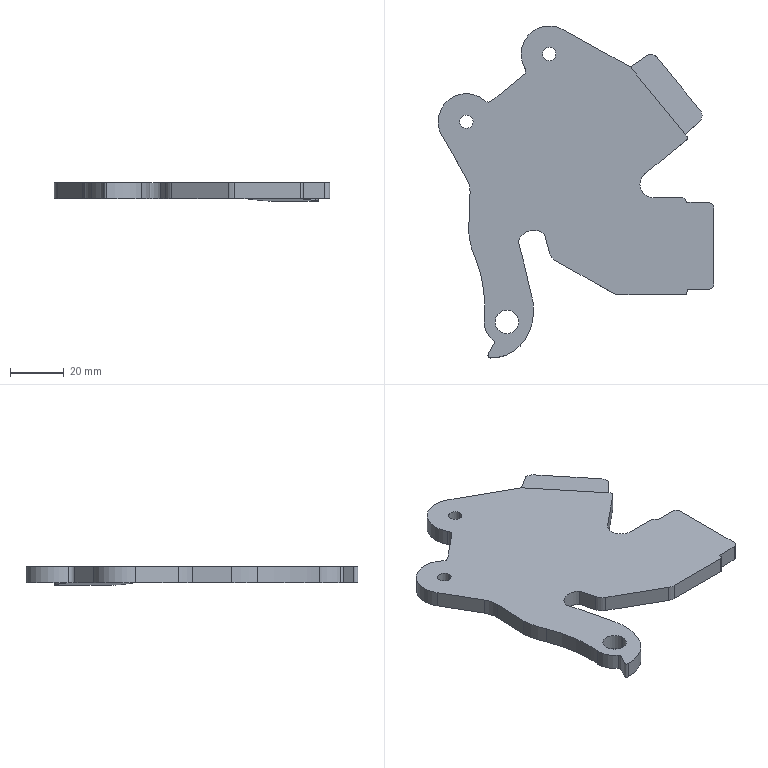Part | STEP file | PRT0001_68_4 | 1 solid | 54 faces | box 102.996 x 124.109 x 6.875 mm | volume 43677 mm3 | cylinder 29 | plane 25 | commonest cylinder face diameters 4 x5 2 x4 5 x4 10 x3 6 x2 8.8 x2